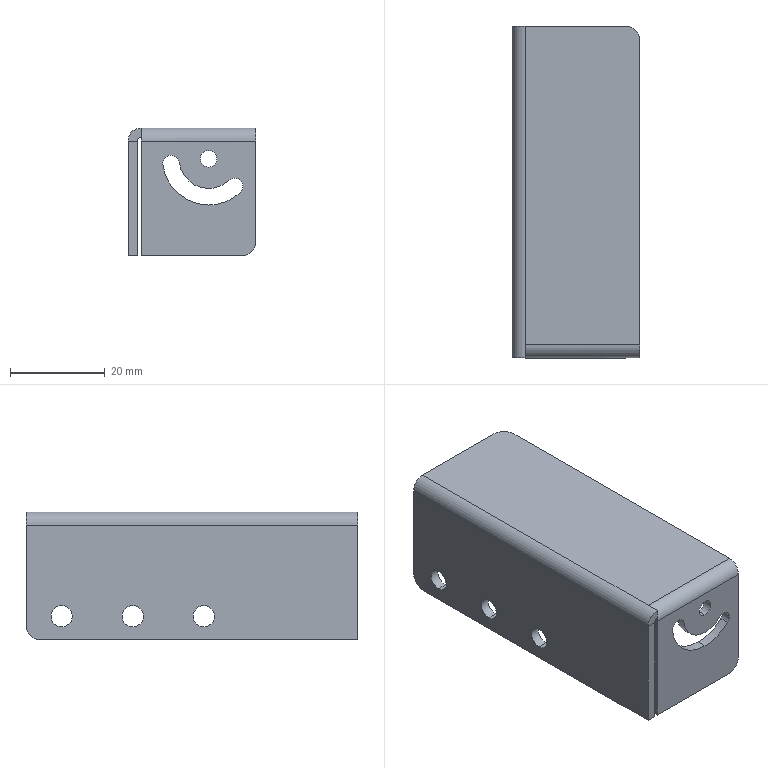Part | SolidWorks | features HoleWzd 2, EdgeFlange 1, Fillet 1, FlatPattern 1, ICE 1, SMBaseFlange 1, SheetMetal 1 | 1 solid | 40 faces | box 27 x 70 x 27 mm | volume 8082 mm3 | cylinder 21 | plane 19 | commonest cylinder face diameters 4.5 x6 3.5 x4 6 x3 1.5 x2 5.5 x2 12.5 x2
STEP:
#1=CARTESIAN_POINT('',(15.,2.,-14.25));
#2=VERTEX_POINT('',#1);
#3=CARTESIAN_POINT('',(21.703,2.,-11.58));
#4=VERTEX_POINT('',#3);
#5=CARTESIAN_POINT('',(15.,2.,-4.5));
#6=DIRECTION('',(0.,-1.,0.));
#7=DIRECTION('',(0.,0.,-1.));
#8=AXIS2_PLACEMENT_3D('',#5,#6,#7);
#9=CIRCLE('',#8,9.75);
#10=EDGE_CURVE('',#2,#4,#9,.T.);
#11=ORIENTED_EDGE('',*,*,#10,.F.);
#12=CARTESIAN_POINT('',(15.,0.,-14.25));
#13=VERTEX_POINT('',#12);
#14=CARTESIAN_POINT('',(15.,2.,-14.25));
#15=DIRECTION('',(0.,-1.,0.));
#16=VECTOR('',#15,1000.);
#17=LINE('',#14,#16);
#18=EDGE_CURVE('',#2,#13,#17,.T.);
#19=ORIENTED_EDGE('',*,*,#18,.T.);
#20=CARTESIAN_POINT('',(21.703,0.,-11.58));
#21=VERTEX_POINT('',#20);
#22=CARTESIAN_POINT('',(15.,0.,-4.5));
#23=DIRECTION('',(0.,-1.,0.));
#24=DIRECTION('',(0.,0.,-1.));
#25=AXIS2_PLACEMENT_3D('',#22,#23,#24);
#26=CIRCLE('',#25,9.75);
#27=EDGE_CURVE('',#13,#21,#26,.T.);
#28=ORIENTED_EDGE('',*,*,#27,.T.);
#29=CARTESIAN_POINT('',(21.703,2.,-11.58));
#30=DIRECTION('',(0.,-1.,0.));
#31=VECTOR('',#30,1000.);
#32=LINE('',#29,#31);
#33=EDGE_CURVE('',#4,#21,#32,.T.);
#34=ORIENTED_EDGE('',*,*,#33,.F.);
#35=EDGE_LOOP('',(#11,#19,#28,#34));
#36=FACE_OUTER_BOUND('',#35,.T.);
#37=CARTESIAN_POINT('',(15.,2.,-4.5));
#38=DIRECTION('',(0.,-1.,0.));
#39=DIRECTION('',(0.,0.,-1.));
#40=AXIS2_PLACEMENT_3D('',#37,#38,#39);
#41=CYLINDRICAL_SURFACE('',#40,9.75);
#42=ADVANCED_FACE('',(#36),#41,.F.);
#43=CARTESIAN_POINT('',(15.,2.,-10.75));
#44=VERTEX_POINT('',#43);
#45=CARTESIAN_POINT('',(8.799,2.,-5.281));
#46=VERTEX_POINT('',#45);
#47=CARTESIAN_POINT('',(15.,2.,-4.5));
#48=DIRECTION('',(0.,1.,0.));
#49=DIRECTION('',(0.,0.,-1.));
#50=AXIS2_PLACEMENT_3D('',#47,#48,#49);
#51=CIRCLE('',#50,6.25);
#52=EDGE_CURVE('',#44,#46,#51,.T.);
#53=ORIENTED_EDGE('',*,*,#52,.F.);
#54=CARTESIAN_POINT('',(15.,0.,-10.75));
#55=VERTEX_POINT('',#54);
#56=CARTESIAN_POINT('',(15.,2.,-10.75));
#57=DIRECTION('',(0.,-1.,0.));
#58=VECTOR('',#57,1000.);
#59=LINE('',#56,#58);
#60=EDGE_CURVE('',#44,#55,#59,.T.);
#61=ORIENTED_EDGE('',*,*,#60,.T.);
#62=CARTESIAN_POINT('',(8.799,0.,-5.281));
#63=VERTEX_POINT('',#62);
#64=CARTESIAN_POINT('',(15.,0.,-4.5));
#65=DIRECTION('',(0.,1.,0.));
#66=DIRECTION('',(0.,0.,-1.));
#67=AXIS2_PLACEMENT_3D('',#64,#65,#66);
#68=CIRCLE('',#67,6.25);
#69=EDGE_CURVE('',#55,#63,#68,.T.);
#70=ORIENTED_EDGE('',*,*,#69,.T.);
#71=CARTESIAN_POINT('',(8.799,2.,-5.281));
#72=DIRECTION('',(0.,-1.,0.));
#73=VECTOR('',#72,1000.);
#74=LINE('',#71,#73);
#75=EDGE_CURVE('',#46,#63,#74,.T.);
#76=ORIENTED_EDGE('',*,*,#75,.F.);
#77=EDGE_LOOP('',(#53,#61,#70,#76));
#78=FACE_OUTER_BOUND('',#77,.T.);
#79=CARTESIAN_POINT('',(15.,2.,-4.5));
#80=DIRECTION('',(0.,-1.,0.));
#81=DIRECTION('',(0.,0.,-1.));
#82=AXIS2_PLACEMENT_3D('',#79,#80,#81);
#83=CYLINDRICAL_SURFACE('',#82,6.25);
#84=ADVANCED_FACE('',(#78),#83,.T.);
#85=CARTESIAN_POINT('',(-2.,62.5,-17.75));
#86=VERTEX_POINT('',#85);
#87=CARTESIAN_POINT('',(-2.,62.5,-22.25));
#88=VERTEX_POINT('',#87);
#89=CARTESIAN_POINT('',(-2.,62.5,-20.));
#90=DIRECTION('',(1.,0.,0.));
#91=DIRECTION('',(0.,0.,-1.));
#92=AXIS2_PLACEMENT_3D('',#89,#90,#91);
#93=CIRCLE('',#92,2.25);
#94=EDGE_CURVE('',#86,#88,#93,.T.);
#95=ORIENTED_EDGE('',*,*,#94,.F.);
#96=CARTESIAN_POINT('',(0.,62.5,-17.75));
#97=VERTEX_POINT('',#96);
#98=CARTESIAN_POINT('',(0.,62.5,-17.75));
#99=DIRECTION('',(1.,0.,0.));
#100=VECTOR('',#99,1000.);
#101=LINE('',#98,#100);
#102=EDGE_CURVE('',#86,#97,#101,.T.);
#103=ORIENTED_EDGE('',*,*,#102,.T.);
#104=CARTESIAN_POINT('',(0.,62.5,-22.25));
#105=VERTEX_POINT('',#104);
#106=CARTESIAN_POINT('',(0.,62.5,-20.));
#107=DIRECTION('',(1.,0.,0.));
#108=DIRECTION('',(0.,0.,-1.));
#109=AXIS2_PLACEMENT_3D('',#106,#107,#108);
#110=CIRCLE('',#109,2.25);
#111=EDGE_CURVE('',#97,#105,#110,.T.);
#112=ORIENTED_EDGE('',*,*,#111,.T.);
#113=CARTESIAN_POINT('',(0.,62.5,-22.25));
#114=DIRECTION('',(1.,0.,0.));
#115=VECTOR('',#114,1000.);
#116=LINE('',#113,#115);
#117=EDGE_CURVE('',#88,#105,#116,.T.);
#118=ORIENTED_EDGE('',*,*,#117,.F.);
#119=EDGE_LOOP('',(#95,#103,#112,#118));
#120=FACE_OUTER_BOUND('',#119,.T.);
#121=CARTESIAN_POINT('',(0.,62.5,-20.));
#122=DIRECTION('',(1.,0.,0.));
#123=DIRECTION('',(0.,0.,-1.));
#124=AXIS2_PLACEMENT_3D('',#121,#122,#123);
#125=CYLINDRICAL_SURFACE('',#124,2.25);
#126=ADVANCED_FACE('',(#120),#125,.F.);
#127=CARTESIAN_POINT('',(-2.,47.5,-17.75));
#128=VERTEX_POINT('',#127);
#129=CARTESIAN_POINT('',(-2.,47.5,-22.25));
#130=VERTEX_POINT('',#129);
#131=CARTESIAN_POINT('',(-2.,47.5,-20.));
#132=DIRECTION('',(1.,0.,0.));
#133=DIRECTION('',(0.,0.,-1.));
#134=AXIS2_PLACEMENT_3D('',#131,#132,#133);
#135=CIRCLE('',#134,2.25);
#136=EDGE_CURVE('',#128,#130,#135,.T.);
#137=ORIENTED_EDGE('',*,*,#136,.F.);
#138=CARTESIAN_POINT('',(0.,47.5,-17.75));
#139=VERTEX_POINT('',#138);
#140=CARTESIAN_POINT('',(0.,47.5,-17.75));
#141=DIRECTION('',(1.,0.,0.));
#142=VECTOR('',#141,1000.);
#143=LINE('',#140,#142);
#144=EDGE_CURVE('',#128,#139,#143,.T.);
#145=ORIENTED_EDGE('',*,*,#144,.T.);
#146=CARTESIAN_POINT('',(0.,47.5,-22.25));
#147=VERTEX_POINT('',#146);
#148=CARTESIAN_POINT('',(0.,47.5,-20.));
#149=DIRECTION('',(1.,0.,0.));
#150=DIRECTION('',(0.,0.,-1.));
#151=AXIS2_PLACEMENT_3D('',#148,#149,#150);
#152=CIRCLE('',#151,2.25);
#153=EDGE_CURVE('',#139,#147,#152,.T.);
#154=ORIENTED_EDGE('',*,*,#153,.T.);
#155=CARTESIAN_POINT('',(0.,47.5,-22.25));
#156=DIRECTION('',(1.,0.,0.));
#157=VECTOR('',#156,1000.);
#158=LINE('',#155,#157);
#159=EDGE_CURVE('',#130,#147,#158,.T.);
#160=ORIENTED_EDGE('',*,*,#159,.F.);
#161=EDGE_LOOP('',(#137,#145,#154,#160));
#162=FACE_OUTER_BOUND('',#161,.T.);
#163=CARTESIAN_POINT('',(0.,47.5,-20.));
#164=DIRECTION('',(1.,0.,0.));
#165=DIRECTION('',(0.,0.,-1.));
#166=AXIS2_PLACEMENT_3D('',#163,#164,#165);
#167=CYLINDRICAL_SURFACE('',#166,2.25);
#168=ADVANCED_FACE('',(#162),#167,.F.);
#169=CARTESIAN_POINT('',(-2.,32.5,-17.75));
#170=VERTEX_POINT('',#169);
#171=CARTESIAN_POINT('',(-2.,32.5,-22.25));
#172=VERTEX_POINT('',#171);
#173=CARTESIAN_POINT('',(-2.,32.5,-20.));
#174=DIRECTION('',(1.,0.,0.));
#175=DIRECTION('',(0.,0.,-1.));
#176=AXIS2_PLACEMENT_3D('',#173,#174,#175);
#177=CIRCLE('',#176,2.25);
#178=EDGE_CURVE('',#170,#172,#177,.T.);
#179=ORIENTED_EDGE('',*,*,#178,.F.);
#180=CARTESIAN_POINT('',(0.,32.5,-17.75));
#181=VERTEX_POINT('',#180);
#182=CARTESIAN_POINT('',(0.,32.5,-17.75));
#183=DIRECTION('',(1.,0.,0.));
#184=VECTOR('',#183,1000.);
#185=LINE('',#182,#184);
#186=EDGE_CURVE('',#170,#181,#185,.T.);
#187=ORIENTED_EDGE('',*,*,#186,.T.);
#188=CARTESIAN_POINT('',(0.,32.5,-22.25));
#189=VERTEX_POINT('',#188);
#190=CARTESIAN_POINT('',(0.,32.5,-20.));
#191=DIRECTION('',(1.,0.,0.));
#192=DIRECTION('',(0.,0.,-1.));
#193=AXIS2_PLACEMENT_3D('',#190,#191,#192);
#194=CIRCLE('',#193,2.25);
#195=EDGE_CURVE('',#181,#189,#194,.T.);
#196=ORIENTED_EDGE('',*,*,#195,.T.);
#197=CARTESIAN_POINT('',(0.,32.5,-22.25));
#198=DIRECTION('',(1.,0.,0.));
#199=VECTOR('',#198,1000.);
#200=LINE('',#197,#199);
#201=EDGE_CURVE('',#172,#189,#200,.T.);
#202=ORIENTED_EDGE('',*,*,#201,.F.);
#203=EDGE_LOOP('',(#179,#187,#196,#202));
#204=FACE_OUTER_BOUND('',#203,.T.);
#205=CARTESIAN_POINT('',(0.,32.5,-20.));
#206=DIRECTION('',(1.,0.,0.));
#207=DIRECTION('',(0.,0.,-1.));
#208=AXIS2_PLACEMENT_3D('',#205,#206,#207);
#209=CYLINDRICAL_SURFACE('',#208,2.25);
#210=ADVANCED_FACE('',(#204),#209,.F.);
#211=CARTESIAN_POINT('',(15.,0.,-2.75));
#212=VERTEX_POINT('',#211);
#213=CARTESIAN_POINT('',(15.,0.,-6.25));
#214=VERTEX_POINT('',#213);
#215=CARTESIAN_POINT('',(15.,0.,-4.5));
#216=DIRECTION('',(0.,-1.,0.));
#217=DIRECTION('',(0.,0.,-1.));
#218=AXIS2_PLACEMENT_3D('',#215,#216,#217);
#219=CIRCLE('',#218,1.75);
#220=EDGE_CURVE('',#212,#214,#219,.T.);
#221=ORIENTED_EDGE('',*,*,#220,.T.);
#222=CARTESIAN_POINT('',(15.,2.,-6.25));
#223=VERTEX_POINT('',#222);
#224=CARTESIAN_POINT('',(15.,2.,-6.25));
#225=DIRECTION('',(0.,1.,0.));
#226=VECTOR('',#225,1000.);
#227=LINE('',#224,#226);
#228=EDGE_CURVE('',#214,#223,#227,.T.);
#229=ORIENTED_EDGE('',*,*,#228,.T.);
#230=CARTESIAN_POINT('',(15.,2.,-2.75));
#231=VERTEX_POINT('',#230);
#232=CARTESIAN_POINT('',(15.,2.,-4.5));
#233=DIRECTION('',(0.,1.,0.));
#234=DIRECTION('',(0.,0.,1.));
#235=AXIS2_PLACEMENT_3D('',#232,#233,#234);
#236=CIRCLE('',#235,1.75);
#237=EDGE_CURVE('',#223,#231,#236,.T.);
#238=ORIENTED_EDGE('',*,*,#237,.T.);
#239=CARTESIAN_POINT('',(15.,2.,-2.75));
#240=DIRECTION('',(0.,1.,0.));
#241=VECTOR('',#240,1000.);
#242=LINE('',#239,#241);
#243=EDGE_CURVE('',#212,#231,#242,.T.);
#244=ORIENTED_EDGE('',*,*,#243,.F.);
#245=EDGE_LOOP('',(#221,#229,#238,#244));
#246=FACE_OUTER_BOUND('',#245,.T.);
#247=CARTESIAN_POINT('',(15.,2.,-4.5));
#248=DIRECTION('',(0.,1.,0.));
#249=DIRECTION('',(0.,0.,1.));
#250=AXIS2_PLACEMENT_3D('',#247,#248,#249);
#251=CYLINDRICAL_SURFACE('',#250,1.75);
#252=ADVANCED_FACE('',(#246),#251,.F.);
#253=CARTESIAN_POINT('',(0.75,0.,0.));
#254=VERTEX_POINT('',#253);
#255=CARTESIAN_POINT('',(0.75,0.1042,0.));
#256=VERTEX_POINT('',#255);
#257=CARTESIAN_POINT('',(0.75,0.,0.));
#258=DIRECTION('',(0.,1.,0.));
#259=VECTOR('',#258,1000.);
#260=LINE('',#257,#259);
#261=EDGE_CURVE('',#254,#256,#260,.T.);
#262=ORIENTED_EDGE('',*,*,#261,.T.);
#263=CARTESIAN_POINT('',(0.75,2.75,2.));
#264=VERTEX_POINT('',#263);
#265=CARTESIAN_POINT('',(0.75,2.75,-0.75));
#266=DIRECTION('',(-1.,0.,0.));
#267=DIRECTION('',(0.,0.,1.));
#268=AXIS2_PLACEMENT_3D('',#265,#266,#267);
#269=CIRCLE('',#268,2.75);
#270=EDGE_CURVE('',#256,#264,#269,.T.);
#271=ORIENTED_EDGE('',*,*,#270,.T.);
#272=CARTESIAN_POINT('',(0.75,0.,2.));
#273=VERTEX_POINT('',#272);
#274=CARTESIAN_POINT('',(0.75,70.,2.));
#275=DIRECTION('',(0.,-1.,0.));
#276=VECTOR('',#275,1000.);
#277=LINE('',#274,#276);
#278=EDGE_CURVE('',#264,#273,#277,.T.);
#279=ORIENTED_EDGE('',*,*,#278,.T.);
#280=CARTESIAN_POINT('',(0.75,0.,2.));
#281=DIRECTION('',(0.,0.,-1.));
#282=VECTOR('',#281,1000.);
#283=LINE('',#280,#282);
#284=EDGE_CURVE('',#273,#254,#283,.T.);
#285=ORIENTED_EDGE('',*,*,#284,.T.);
#286=EDGE_LOOP('',(#262,#271,#279,#285));
#287=FACE_OUTER_BOUND('',#286,.T.);
#288=CARTESIAN_POINT('',(0.75,0.,0.));
#289=DIRECTION('',(1.,0.,0.));
#290=DIRECTION('',(0.,1.,0.));
#291=AXIS2_PLACEMENT_3D('',#288,#289,#290);
#292=PLANE('',#291);
#293=ADVANCED_FACE('',(#287),#292,.T.);
#294=CARTESIAN_POINT('',(25.,67.,2.));
#295=VERTEX_POINT('',#294);
#296=CARTESIAN_POINT('',(25.,2.75,2.));
#297=VERTEX_POINT('',#296);
#298=CARTESIAN_POINT('',(25.,70.,2.));
#299=DIRECTION('',(0.,-1.,0.));
#300=VECTOR('',#299,1000.);
#301=LINE('',#298,#300);
#302=EDGE_CURVE('',#295,#297,#301,.T.);
#303=ORIENTED_EDGE('',*,*,#302,.F.);
#304=CARTESIAN_POINT('',(22.,70.,2.));
#305=VERTEX_POINT('',#304);
#306=CARTESIAN_POINT('',(22.,67.,2.));
#307=DIRECTION('',(0.,0.,1.));
#308=DIRECTION('',(-1.,0.,0.));
#309=AXIS2_PLACEMENT_3D('',#306,#307,#308);
#310=CIRCLE('',#309,3.);
#311=EDGE_CURVE('',#295,#305,#310,.T.);
#312=ORIENTED_EDGE('',*,*,#311,.T.);
#313=CARTESIAN_POINT('',(0.75,70.,2.));
#314=VERTEX_POINT('',#313);
#315=CARTESIAN_POINT('',(0.,70.,2.));
#316=DIRECTION('',(1.,0.,0.));
#317=VECTOR('',#316,1000.);
#318=LINE('',#315,#317);
#319=EDGE_CURVE('',#314,#305,#318,.T.);
#320=ORIENTED_EDGE('',*,*,#319,.F.);
#321=CARTESIAN_POINT('',(0.75,70.,2.));
#322=DIRECTION('',(0.,-1.,0.));
#323=VECTOR('',#322,1000.);
#324=LINE('',#321,#323);
#325=EDGE_CURVE('',#314,#264,#324,.T.);
#326=ORIENTED_EDGE('',*,*,#325,.T.);
#327=CARTESIAN_POINT('',(0.75,2.75,2.));
#328=DIRECTION('',(1.,0.,0.));
#329=VECTOR('',#328,1000.);
#330=LINE('',#327,#329);
#331=EDGE_CURVE('',#264,#297,#330,.T.);
#332=ORIENTED_EDGE('',*,*,#331,.T.);
#333=EDGE_LOOP('',(#303,#312,#320,#326,#332));
#334=FACE_OUTER_BOUND('',#333,.T.);
#335=CARTESIAN_POINT('',(0.,70.,2.));
#336=DIRECTION('',(0.,0.,-1.));
#337=DIRECTION('',(-1.,0.,0.));
#338=AXIS2_PLACEMENT_3D('',#335,#336,#337);
#339=PLANE('',#338);
#340=ADVANCED_FACE('',(#334),#339,.F.);
#341=CARTESIAN_POINT('',(0.75,70.,0.));
#342=VERTEX_POINT('',#341);
#343=CARTESIAN_POINT('',(22.,70.,0.));
#344=VERTEX_POINT('',#343);
#345=CARTESIAN_POINT('',(0.,70.,0.));
#346=DIRECTION('',(1.,0.,0.));
#347=VECTOR('',#346,1000.);
#348=LINE('',#345,#347);
#349=EDGE_CURVE('',#342,#344,#348,.T.);
#350=ORIENTED_EDGE('',*,*,#349,.T.);
#351=CARTESIAN_POINT('',(25.,67.,0.));
#352=VERTEX_POINT('',#351);
#353=CARTESIAN_POINT('',(22.,67.,0.));
#354=DIRECTION('',(0.,0.,-1.));
#355=DIRECTION('',(-1.,0.,0.));
#356=AXIS2_PLACEMENT_3D('',#353,#354,#355);
#357=CIRCLE('',#356,3.);
#358=EDGE_CURVE('',#344,#352,#357,.T.);
#359=ORIENTED_EDGE('',*,*,#358,.T.);
#360=CARTESIAN_POINT('',(25.,2.75,0.));
#361=VERTEX_POINT('',#360);
#362=CARTESIAN_POINT('',(25.,70.,0.));
#363=DIRECTION('',(0.,-1.,0.));
#364=VECTOR('',#363,1000.);
#365=LINE('',#362,#364);
#366=EDGE_CURVE('',#352,#361,#365,.T.);
#367=ORIENTED_EDGE('',*,*,#366,.T.);
#368=CARTESIAN_POINT('',(0.75,2.75,0.));
#369=VERTEX_POINT('',#368);
#370=CARTESIAN_POINT('',(0.75,2.75,0.));
#371=DIRECTION('',(1.,0.,0.));
#372=VECTOR('',#371,1000.);
#373=LINE('',#370,#372);
#374=EDGE_CURVE('',#369,#361,#373,.T.);
#375=ORIENTED_EDGE('',*,*,#374,.F.);
#376=CARTESIAN_POINT('',(0.75,70.,0.));
#377=DIRECTION('',(0.,-1.,0.));
#378=VECTOR('',#377,1000.);
#379=LINE('',#376,#378);
#380=EDGE_CURVE('',#342,#369,#379,.T.);
#381=ORIENTED_EDGE('',*,*,#380,.F.);
#382=EDGE_LOOP('',(#350,#359,#367,#375,#381));
#383=FACE_OUTER_BOUND('',#382,.T.);
#384=CARTESIAN_POINT('',(0.,70.,0.));
#385=DIRECTION('',(0.,0.,-1.));
#386=DIRECTION('',(-1.,0.,0.));
#387=AXIS2_PLACEMENT_3D('',#384,#385,#386);
#388=PLANE('',#387);
#389=ADVANCED_FACE('',(#383),#388,.T.);
#390=CARTESIAN_POINT('',(0.75,70.,0.));
#391=DIRECTION('',(0.,0.,1.));
#392=VECTOR('',#391,1000.);
#393=LINE('',#390,#392);
#394=EDGE_CURVE('',#342,#314,#393,.T.);
#395=ORIENTED_EDGE('',*,*,#394,.F.);
#396=CARTESIAN_POINT('',(0.,70.,-0.75));
#397=VERTEX_POINT('',#396);
#398=CARTESIAN_POINT('',(0.75,70.,-0.75));
#399=DIRECTION('',(0.,1.,0.));
#400=DIRECTION('',(0.,0.,-1.));
#401=AXIS2_PLACEMENT_3D('',#398,#399,#400);
#402=CIRCLE('',#401,0.75);
#403=EDGE_CURVE('',#397,#342,#402,.T.);
#404=ORIENTED_EDGE('',*,*,#403,.F.);
#405=CARTESIAN_POINT('',(-2.,70.,-0.75));
#406=VERTEX_POINT('',#405);
#407=CARTESIAN_POINT('',(-2.,70.,-0.75));
#408=DIRECTION('',(1.,0.,0.));
#409=VECTOR('',#408,1000.);
#410=LINE('',#407,#409);
#411=EDGE_CURVE('',#406,#397,#410,.T.);
#412=ORIENTED_EDGE('',*,*,#411,.F.);
#413=CARTESIAN_POINT('',(0.75,70.,-0.75));
#414=DIRECTION('',(0.,1.,0.));
#415=DIRECTION('',(1.,0.,0.));
#416=AXIS2_PLACEMENT_3D('',#413,#414,#415);
#417=CIRCLE('',#416,2.75);
#418=EDGE_CURVE('',#406,#314,#417,.T.);
#419=ORIENTED_EDGE('',*,*,#418,.T.);
#420=EDGE_LOOP('',(#395,#404,#412,#419));
#421=FACE_OUTER_BOUND('',#420,.T.);
#422=CARTESIAN_POINT('',(0.75,70.,0.));
#423=DIRECTION('',(0.,1.,0.));
#424=DIRECTION('',(0.,0.,1.));
#425=AXIS2_PLACEMENT_3D('',#422,#423,#424);
#426=PLANE('',#425);
#427=ADVANCED_FACE('',(#421),#426,.T.);
#428=ORIENTED_EDGE('',*,*,#319,.T.);
#429=CARTESIAN_POINT('',(22.,70.,-0.75));
#430=DIRECTION('',(0.,0.,-1.));
#431=VECTOR('',#430,1000.);
#432=LINE('',#429,#431);
#433=EDGE_CURVE('',#305,#344,#432,.T.);
#434=ORIENTED_EDGE('',*,*,#433,.T.);
#435=ORIENTED_EDGE('',*,*,#349,.F.);
#436=ORIENTED_EDGE('',*,*,#394,.T.);
#437=EDGE_LOOP('',(#428,#434,#435,#436));
#438=FACE_OUTER_BOUND('',#437,.T.);
#439=CARTESIAN_POINT('',(-2.,70.,-0.75));
#440=DIRECTION('',(0.,1.,0.));
#441=DIRECTION('',(0.,0.,1.));
#442=AXIS2_PLACEMENT_3D('',#439,#440,#441);
#443=PLANE('',#442);
#444=ADVANCED_FACE('',(#438),#443,.T.);
#445=CARTESIAN_POINT('',(0.,0.,-0.75));
#446=VERTEX_POINT('',#445);
#447=CARTESIAN_POINT('',(-2.,0.,-0.75));
#448=VERTEX_POINT('',#447);
#449=CARTESIAN_POINT('',(0.,0.,-0.75));
#450=DIRECTION('',(-1.,0.,0.));
#451=VECTOR('',#450,1000.);
#452=LINE('',#449,#451);
#453=EDGE_CURVE('',#446,#448,#452,.T.);
#454=ORIENTED_EDGE('',*,*,#453,.F.);
#455=CARTESIAN_POINT('',(0.75,0.,-0.75));
#456=DIRECTION('',(0.,1.,0.));
#457=DIRECTION('',(0.,0.,-1.));
#458=AXIS2_PLACEMENT_3D('',#455,#456,#457);
#459=CIRCLE('',#458,0.75);
#460=EDGE_CURVE('',#446,#254,#459,.T.);
#461=ORIENTED_EDGE('',*,*,#460,.T.);
#462=ORIENTED_EDGE('',*,*,#284,.F.);
#463=CARTESIAN_POINT('',(0.75,0.,-0.75));
#464=DIRECTION('',(0.,1.,0.));
#465=DIRECTION('',(1.,0.,0.));
#466=AXIS2_PLACEMENT_3D('',#463,#464,#465);
#467=CIRCLE('',#466,2.75);
#468=EDGE_CURVE('',#448,#273,#467,.T.);
#469=ORIENTED_EDGE('',*,*,#468,.F.);
#470=EDGE_LOOP('',(#454,#461,#462,#469));
#471=FACE_OUTER_BOUND('',#470,.T.);
#472=CARTESIAN_POINT('',(0.,0.,-0.75));
#473=DIRECTION('',(0.,-1.,0.));
#474=DIRECTION('',(0.,0.,-1.));
#475=AXIS2_PLACEMENT_3D('',#472,#473,#474);
#476=PLANE('',#475);
#477=ADVANCED_FACE('',(#471),#476,.T.);
#478=CARTESIAN_POINT('',(0.,0.,-25.));
#479=VERTEX_POINT('',#478);
#480=CARTESIAN_POINT('',(0.,0.,-25.));
#481=DIRECTION('',(0.,0.,1.));
#482=VECTOR('',#481,1000.);
#483=LINE('',#480,#482);
#484=EDGE_CURVE('',#479,#446,#483,.T.);
#485=ORIENTED_EDGE('',*,*,#484,.T.);
#486=ORIENTED_EDGE('',*,*,#453,.T.);
#487=CARTESIAN_POINT('',(-2.,0.,-25.));
#488=VERTEX_POINT('',#487);
#489=CARTESIAN_POINT('',(-2.,0.,-25.));
#490=DIRECTION('',(0.,0.,1.));
#491=VECTOR('',#490,1000.);
#492=LINE('',#489,#491);
#493=EDGE_CURVE('',#488,#448,#492,.T.);
#494=ORIENTED_EDGE('',*,*,#493,.F.);
#495=CARTESIAN_POINT('',(-2.,0.,-25.));
#496=DIRECTION('',(1.,0.,0.));
#497=VECTOR('',#496,1000.);
#498=LINE('',#495,#497);
#499=EDGE_CURVE('',#488,#479,#498,.T.);
#500=ORIENTED_EDGE('',*,*,#499,.T.);
#501=EDGE_LOOP('',(#485,#486,#494,#500));
#502=FACE_OUTER_BOUND('',#501,.T.);
#503=CARTESIAN_POINT('',(0.75,0.,2.));
#504=DIRECTION('',(0.,-1.,0.));
#505=DIRECTION('',(0.,0.,-1.));
#506=AXIS2_PLACEMENT_3D('',#503,#504,#505);
#507=PLANE('',#506);
#508=ADVANCED_FACE('',(#502),#507,.T.);
#509=ORIENTED_EDGE('',*,*,#366,.F.);
#510=CARTESIAN_POINT('',(25.,67.,0.));
#511=DIRECTION('',(0.,0.,1.));
#512=VECTOR('',#511,1000.);
#513=LINE('',#510,#512);
#514=EDGE_CURVE('',#352,#295,#513,.T.);
#515=ORIENTED_EDGE('',*,*,#514,.T.);
#516=ORIENTED_EDGE('',*,*,#302,.T.);
#517=CARTESIAN_POINT('',(25.,2.75,0.));
#518=DIRECTION('',(0.,0.,1.));
#519=VECTOR('',#518,1000.);
#520=LINE('',#517,#519);
#521=EDGE_CURVE('',#361,#297,#520,.T.);
#522=ORIENTED_EDGE('',*,*,#521,.F.);
#523=EDGE_LOOP('',(#509,#515,#516,#522));
#524=FACE_OUTER_BOUND('',#523,.T.);
#525=CARTESIAN_POINT('',(25.,70.,0.));
#526=DIRECTION('',(1.,0.,0.));
#527=DIRECTION('',(0.,0.,-1.));
#528=AXIS2_PLACEMENT_3D('',#525,#526,#527);
#529=PLANE('',#528);
#530=ADVANCED_FACE('',(#524),#529,.T.);
#531=ORIENTED_EDGE('',*,*,#460,.F.);
#532=CARTESIAN_POINT('',(0.,70.,-0.75));
#533=DIRECTION('',(0.,-1.,0.));
#534=VECTOR('',#533,1000.);
#535=LINE('',#532,#534);
#536=EDGE_CURVE('',#397,#446,#535,.T.);
#537=ORIENTED_EDGE('',*,*,#536,.F.);
#538=ORIENTED_EDGE('',*,*,#403,.T.);
#539=ORIENTED_EDGE('',*,*,#380,.T.);
#540=CARTESIAN_POINT('',(0.75,0.,0.));
#541=DIRECTION('',(0.,1.,0.));
#542=VECTOR('',#541,1000.);
#543=LINE('',#540,#542);
#544=EDGE_CURVE('',#256,#369,#543,.T.);
#545=ORIENTED_EDGE('',*,*,#544,.F.);
#546=ORIENTED_EDGE('',*,*,#261,.F.);
#547=EDGE_LOOP('',(#531,#537,#538,#539,#545,#546));
#548=FACE_OUTER_BOUND('',#547,.T.);
#549=CARTESIAN_POINT('',(0.75,70.,-0.75));
#550=DIRECTION('',(0.,-1.,0.));
#551=DIRECTION('',(0.,0.,-1.));
#552=AXIS2_PLACEMENT_3D('',#549,#550,#551);
#553=CYLINDRICAL_SURFACE('',#552,0.75);
#554=ADVANCED_FACE('',(#548),#553,.F.);
#555=CARTESIAN_POINT('',(0.,62.5,-20.));
#556=DIRECTION('',(1.,0.,0.));
#557=DIRECTION('',(0.,0.,-1.));
#558=AXIS2_PLACEMENT_3D('',#555,#556,#557);
#559=CIRCLE('',#558,2.25);
#560=EDGE_CURVE('',#105,#97,#559,.T.);
#561=ORIENTED_EDGE('',*,*,#560,.F.);
#562=ORIENTED_EDGE('',*,*,#111,.F.);
#563=EDGE_LOOP('',(#561,#562));
#564=FACE_BOUND('',#563,.T.);
#565=CARTESIAN_POINT('',(0.,47.5,-20.));
#566=DIRECTION('',(1.,0.,0.));
#567=DIRECTION('',(0.,0.,-1.));
#568=AXIS2_PLACEMENT_3D('',#565,#566,#567);
#569=CIRCLE('',#568,2.25);
#570=EDGE_CURVE('',#147,#139,#569,.T.);
#571=ORIENTED_EDGE('',*,*,#570,.F.);
#572=ORIENTED_EDGE('',*,*,#153,.F.);
#573=EDGE_LOOP('',(#571,#572));
#574=FACE_BOUND('',#573,.T.);
#575=CARTESIAN_POINT('',(0.,32.5,-20.));
#576=DIRECTION('',(1.,0.,0.));
#577=DIRECTION('',(0.,0.,-1.));
#578=AXIS2_PLACEMENT_3D('',#575,#576,#577);
#579=CIRCLE('',#578,2.25);
#580=EDGE_CURVE('',#189,#181,#579,.T.);
#581=ORIENTED_EDGE('',*,*,#580,.F.);
#582=ORIENTED_EDGE('',*,*,#195,.F.);
#583=EDGE_LOOP('',(#581,#582));
#584=FACE_BOUND('',#583,.T.);
#585=CARTESIAN_POINT('',(0.,67.,-25.));
#586=VERTEX_POINT('',#585);
#587=CARTESIAN_POINT('',(0.,70.,-25.));
#588=DIRECTION('',(0.,-1.,0.));
#589=VECTOR('',#588,1000.);
#590=LINE('',#587,#589);
#591=EDGE_CURVE('',#586,#479,#590,.T.);
#592=ORIENTED_EDGE('',*,*,#591,.F.);
#593=CARTESIAN_POINT('',(0.,70.,-22.));
#594=VERTEX_POINT('',#593);
#595=CARTESIAN_POINT('',(0.,67.,-22.));
#596=DIRECTION('',(1.,0.,0.));
#597=DIRECTION('',(0.,0.,-1.));
#598=AXIS2_PLACEMENT_3D('',#595,#596,#597);
#599=CIRCLE('',#598,3.);
#600=EDGE_CURVE('',#586,#594,#599,.T.);
#601=ORIENTED_EDGE('',*,*,#600,.T.);
#602=CARTESIAN_POINT('',(0.,70.,-25.));
#603=DIRECTION('',(0.,0.,1.));
#604=VECTOR('',#603,1000.);
#605=LINE('',#602,#604);
#606=EDGE_CURVE('',#594,#397,#605,.T.);
#607=ORIENTED_EDGE('',*,*,#606,.T.);
#608=ORIENTED_EDGE('',*,*,#536,.T.);
#609=ORIENTED_EDGE('',*,*,#484,.F.);
#610=EDGE_LOOP('',(#592,#601,#607,#608,#609));
#611=FACE_OUTER_BOUND('',#610,.T.);
#612=CARTESIAN_POINT('',(0.,70.,-25.));
#613=DIRECTION('',(1.,0.,0.));
#614=DIRECTION('',(0.,0.,-1.));
#615=AXIS2_PLACEMENT_3D('',#612,#613,#614);
#616=PLANE('',#615);
#617=ADVANCED_FACE('',(#564,#574,#584,#611),#616,.T.);
#618=CARTESIAN_POINT('',(-2.,67.,-25.));
#619=VERTEX_POINT('',#618);
#620=CARTESIAN_POINT('',(-2.,70.,-25.));
#621=DIRECTION('',(0.,-1.,0.));
#622=VECTOR('',#621,1000.);
#623=LINE('',#620,#622);
#624=EDGE_CURVE('',#619,#488,#623,.T.);
#625=ORIENTED_EDGE('',*,*,#624,.F.);
#626=CARTESIAN_POINT('',(0.,67.,-25.));
#627=DIRECTION('',(1.,0.,0.));
#628=VECTOR('',#627,1000.);
#629=LINE('',#626,#628);
#630=EDGE_CURVE('',#619,#586,#629,.T.);
#631=ORIENTED_EDGE('',*,*,#630,.T.);
#632=ORIENTED_EDGE('',*,*,#591,.T.);
#633=ORIENTED_EDGE('',*,*,#499,.F.);
#634=EDGE_LOOP('',(#625,#631,#632,#633));
#635=FACE_OUTER_BOUND('',#634,.T.);
#636=CARTESIAN_POINT('',(-2.,70.,-25.));
#637=DIRECTION('',(0.,0.,-1.));
#638=DIRECTION('',(-1.,0.,0.));
#639=AXIS2_PLACEMENT_3D('',#636,#637,#638);
#640=PLANE('',#639);
#641=ADVANCED_FACE('',(#635),#640,.T.);
#642=CARTESIAN_POINT('',(-2.,62.5,-20.));
#643=DIRECTION('',(1.,0.,0.));
#644=DIRECTION('',(0.,0.,-1.));
#645=AXIS2_PLACEMENT_3D('',#642,#643,#644);
#646=CIRCLE('',#645,2.25);
#647=EDGE_CURVE('',#88,#86,#646,.T.);
#648=ORIENTED_EDGE('',*,*,#647,.T.);
#649=ORIENTED_EDGE('',*,*,#94,.T.);
#650=EDGE_LOOP('',(#648,#649));
#651=FACE_BOUND('',#650,.T.);
#652=CARTESIAN_POINT('',(-2.,47.5,-20.));
#653=DIRECTION('',(1.,0.,0.));
#654=DIRECTION('',(0.,0.,-1.));
#655=AXIS2_PLACEMENT_3D('',#652,#653,#654);
#656=CIRCLE('',#655,2.25);
#657=EDGE_CURVE('',#130,#128,#656,.T.);
#658=ORIENTED_EDGE('',*,*,#657,.T.);
#659=ORIENTED_EDGE('',*,*,#136,.T.);
#660=EDGE_LOOP('',(#658,#659));
#661=FACE_BOUND('',#660,.T.);
#662=CARTESIAN_POINT('',(-2.,32.5,-20.));
#663=DIRECTION('',(1.,0.,0.));
#664=DIRECTION('',(0.,0.,-1.));
#665=AXIS2_PLACEMENT_3D('',#662,#663,#664);
#666=CIRCLE('',#665,2.25);
#667=EDGE_CURVE('',#172,#170,#666,.T.);
#668=ORIENTED_EDGE('',*,*,#667,.T.);
#669=ORIENTED_EDGE('',*,*,#178,.T.);
#670=EDGE_LOOP('',(#668,#669));
#671=FACE_BOUND('',#670,.T.);
#672=CARTESIAN_POINT('',(-2.,70.,-22.));
#673=VERTEX_POINT('',#672);
#674=CARTESIAN_POINT('',(-2.,70.,-25.));
#675=DIRECTION('',(0.,0.,1.));
#676=VECTOR('',#675,1000.);
#677=LINE('',#674,#676);
#678=EDGE_CURVE('',#673,#406,#677,.T.);
#679=ORIENTED_EDGE('',*,*,#678,.F.);
#680=CARTESIAN_POINT('',(-2.,67.,-22.));
#681=DIRECTION('',(-1.,0.,0.));
#682=DIRECTION('',(0.,0.,-1.));
#683=AXIS2_PLACEMENT_3D('',#680,#681,#682);
#684=CIRCLE('',#683,3.);
#685=EDGE_CURVE('',#673,#619,#684,.T.);
#686=ORIENTED_EDGE('',*,*,#685,.T.);
#687=ORIENTED_EDGE('',*,*,#624,.T.);
#688=ORIENTED_EDGE('',*,*,#493,.T.);
#689=CARTESIAN_POINT('',(-2.,70.,-0.75));
#690=DIRECTION('',(0.,-1.,0.));
#691=VECTOR('',#690,1000.);
#692=LINE('',#689,#691);
#693=EDGE_CURVE('',#406,#448,#692,.T.);
#694=ORIENTED_EDGE('',*,*,#693,.F.);
#695=EDGE_LOOP('',(#679,#686,#687,#688,#694));
#696=FACE_OUTER_BOUND('',#695,.T.);
#697=CARTESIAN_POINT('',(-2.,70.,-25.));
#698=DIRECTION('',(1.,0.,0.));
#699=DIRECTION('',(0.,0.,-1.));
#700=AXIS2_PLACEMENT_3D('',#697,#698,#699);
#701=PLANE('',#700);
#702=ADVANCED_FACE('',(#651,#661,#671,#696),#701,.F.);
#703=ORIENTED_EDGE('',*,*,#468,.T.);
#704=ORIENTED_EDGE('',*,*,#278,.F.);
#705=ORIENTED_EDGE('',*,*,#325,.F.);
#706=ORIENTED_EDGE('',*,*,#418,.F.);
#707=ORIENTED_EDGE('',*,*,#693,.T.);
#708=EDGE_LOOP('',(#703,#704,#705,#706,#707));
#709=FACE_OUTER_BOUND('',#708,.T.);
#710=CARTESIAN_POINT('',(0.75,70.,-0.75));
#711=DIRECTION('',(0.,-1.,0.));
#712=DIRECTION('',(0.,0.,-1.));
#713=AXIS2_PLACEMENT_3D('',#710,#711,#712);
#714=CYLINDRICAL_SURFACE('',#713,2.75);
#715=ADVANCED_FACE('',(#709),#714,.T.);
#716=ORIENTED_EDGE('',*,*,#606,.F.);
#717=CARTESIAN_POINT('',(-2.,70.,-22.));
#718=DIRECTION('',(-1.,0.,0.));
#719=VECTOR('',#718,1000.);
#720=LINE('',#717,#719);
#721=EDGE_CURVE('',#594,#673,#720,.T.);
#722=ORIENTED_EDGE('',*,*,#721,.T.);
#723=ORIENTED_EDGE('',*,*,#678,.T.);
#724=ORIENTED_EDGE('',*,*,#411,.T.);
#725=EDGE_LOOP('',(#716,#722,#723,#724));
#726=FACE_OUTER_BOUND('',#725,.T.);
#727=CARTESIAN_POINT('',(0.75,70.,-0.75));
#728=DIRECTION('',(0.,-1.,0.));
#729=DIRECTION('',(-1.,0.,0.));
#730=AXIS2_PLACEMENT_3D('',#727,#728,#729);
#731=PLANE('',#730);
#732=ADVANCED_FACE('',(#726),#731,.F.);
#733=CARTESIAN_POINT('',(25.,2.,-0.75));
#734=VERTEX_POINT('',#733);
#735=CARTESIAN_POINT('',(25.,0.,-0.75));
#736=VERTEX_POINT('',#735);
#737=CARTESIAN_POINT('',(25.,0.,-0.75));
#738=DIRECTION('',(0.,-1.,0.));
#739=VECTOR('',#738,1000.);
#740=LINE('',#737,#739);
#741=EDGE_CURVE('',#734,#736,#740,.T.);
#742=ORIENTED_EDGE('',*,*,#741,.F.);
#743=CARTESIAN_POINT('',(25.,2.75,-0.75));
#744=DIRECTION('',(1.,0.,0.));
#745=DIRECTION('',(0.,0.,1.));
#746=AXIS2_PLACEMENT_3D('',#743,#744,#745);
#747=CIRCLE('',#746,0.75);
#748=EDGE_CURVE('',#361,#734,#747,.T.);
#749=ORIENTED_EDGE('',*,*,#748,.F.);
#750=ORIENTED_EDGE('',*,*,#521,.T.);
#751=CARTESIAN_POINT('',(25.,2.75,-0.75));
#752=DIRECTION('',(1.,0.,0.));
#753=DIRECTION('',(0.,0.,1.));
#754=AXIS2_PLACEMENT_3D('',#751,#752,#753);
#755=CIRCLE('',#754,2.75);
#756=EDGE_CURVE('',#297,#736,#755,.T.);
#757=ORIENTED_EDGE('',*,*,#756,.T.);
#758=EDGE_LOOP('',(#742,#749,#750,#757));
#759=FACE_OUTER_BOUND('',#758,.T.);
#760=CARTESIAN_POINT('',(25.,2.75,-0.75));
#761=DIRECTION('',(1.,0.,0.));
#762=DIRECTION('',(0.,0.,-1.));
#763=AXIS2_PLACEMENT_3D('',#760,#761,#762);
#764=PLANE('',#763);
#765=ADVANCED_FACE('',(#759),#764,.T.);
#766=CARTESIAN_POINT('',(0.75,0.,-0.75));
#767=VERTEX_POINT('',#766);
#768=CARTESIAN_POINT('',(0.75,2.75,-0.75));
#769=DIRECTION('',(-1.,0.,0.));
#770=DIRECTION('',(0.,0.,1.));
#771=AXIS2_PLACEMENT_3D('',#768,#769,#770);
#772=CIRCLE('',#771,2.75);
#773=EDGE_CURVE('',#767,#256,#772,.T.);
#774=ORIENTED_EDGE('',*,*,#773,.T.);
#775=ORIENTED_EDGE('',*,*,#544,.T.);
#776=CARTESIAN_POINT('',(0.75,2.,-0.75));
#777=VERTEX_POINT('',#776);
#778=CARTESIAN_POINT('',(0.75,2.75,-0.75));
#779=DIRECTION('',(-1.,0.,0.));
#780=DIRECTION('',(0.,0.,1.));
#781=AXIS2_PLACEMENT_3D('',#778,#779,#780);
#782=CIRCLE('',#781,0.75);
#783=EDGE_CURVE('',#777,#369,#782,.T.);
#784=ORIENTED_EDGE('',*,*,#783,.F.);
#785=CARTESIAN_POINT('',(0.75,2.,-0.75));
#786=DIRECTION('',(0.,-1.,0.));
#787=VECTOR('',#786,1000.);
#788=LINE('',#785,#787);
#789=EDGE_CURVE('',#777,#767,#788,.T.);
#790=ORIENTED_EDGE('',*,*,#789,.T.);
#791=EDGE_LOOP('',(#774,#775,#784,#790));
#792=FACE_OUTER_BOUND('',#791,.T.);
#793=CARTESIAN_POINT('',(0.75,2.75,-0.75));
#794=DIRECTION('',(1.,0.,0.));
#795=DIRECTION('',(0.,0.,-1.));
#796=AXIS2_PLACEMENT_3D('',#793,#794,#795);
#797=PLANE('',#796);
#798=ADVANCED_FACE('',(#792),#797,.F.);
#799=ORIENTED_EDGE('',*,*,#331,.F.);
#800=ORIENTED_EDGE('',*,*,#270,.F.);
#801=ORIENTED_EDGE('',*,*,#773,.F.);
#802=CARTESIAN_POINT('',(0.,0.,-0.75));
#803=DIRECTION('',(-1.,0.,0.));
#804=VECTOR('',#803,1000.);
#805=LINE('',#802,#804);
#806=EDGE_CURVE('',#736,#767,#805,.T.);
#807=ORIENTED_EDGE('',*,*,#806,.F.);
#808=ORIENTED_EDGE('',*,*,#756,.F.);
#809=EDGE_LOOP('',(#799,#800,#801,#807,#808));
#810=FACE_OUTER_BOUND('',#809,.T.);
#811=CARTESIAN_POINT('',(0.75,2.75,-0.75));
#812=DIRECTION('',(-1.,0.,0.));
#813=DIRECTION('',(0.,-1.,0.));
#814=AXIS2_PLACEMENT_3D('',#811,#812,#813);
#815=CYLINDRICAL_SURFACE('',#814,2.75);
#816=ADVANCED_FACE('',(#810),#815,.T.);
#817=ORIENTED_EDGE('',*,*,#374,.T.);
#818=ORIENTED_EDGE('',*,*,#748,.T.);
#819=CARTESIAN_POINT('',(25.,2.,-0.75));
#820=DIRECTION('',(-1.,0.,0.));
#821=VECTOR('',#820,1000.);
#822=LINE('',#819,#821);
#823=EDGE_CURVE('',#734,#777,#822,.T.);
#824=ORIENTED_EDGE('',*,*,#823,.T.);
#825=ORIENTED_EDGE('',*,*,#783,.T.);
#826=EDGE_LOOP('',(#817,#818,#824,#825));
#827=FACE_OUTER_BOUND('',#826,.T.);
#828=CARTESIAN_POINT('',(0.75,2.75,-0.75));
#829=DIRECTION('',(-1.,0.,0.));
#830=DIRECTION('',(0.,-1.,0.));
#831=AXIS2_PLACEMENT_3D('',#828,#829,#830);
#832=CYLINDRICAL_SURFACE('',#831,0.75);
#833=ADVANCED_FACE('',(#827),#832,.F.);
#834=CARTESIAN_POINT('',(0.75,0.,-25.));
#835=VERTEX_POINT('',#834);
#836=CARTESIAN_POINT('',(0.75,0.,0.));
#837=DIRECTION('',(0.,0.,1.));
#838=VECTOR('',#837,1000.);
#839=LINE('',#836,#838);
#840=EDGE_CURVE('',#835,#767,#839,.T.);
#841=ORIENTED_EDGE('',*,*,#840,.T.);
#842=ORIENTED_EDGE('',*,*,#789,.F.);
#843=CARTESIAN_POINT('',(0.75,2.,-25.));
#844=VERTEX_POINT('',#843);
#845=CARTESIAN_POINT('',(0.75,2.,0.));
#846=DIRECTION('',(0.,0.,1.));
#847=VECTOR('',#846,1000.);
#848=LINE('',#845,#847);
#849=EDGE_CURVE('',#844,#777,#848,.T.);
#850=ORIENTED_EDGE('',*,*,#849,.F.);
#851=CARTESIAN_POINT('',(0.75,0.,-25.));
#852=DIRECTION('',(0.,1.,0.));
#853=VECTOR('',#852,1000.);
#854=LINE('',#851,#853);
#855=EDGE_CURVE('',#835,#844,#854,.T.);
#856=ORIENTED_EDGE('',*,*,#855,.F.);
#857=EDGE_LOOP('',(#841,#842,#850,#856));
#858=FACE_OUTER_BOUND('',#857,.T.);
#859=CARTESIAN_POINT('',(0.75,0.,0.));
#860=DIRECTION('',(-1.,0.,0.));
#861=DIRECTION('',(0.,0.,1.));
#862=AXIS2_PLACEMENT_3D('',#859,#860,#861);
#863=PLANE('',#862);
#864=ADVANCED_FACE('',(#858),#863,.T.);
#865=CARTESIAN_POINT('',(25.,0.,-22.));
#866=VERTEX_POINT('',#865);
#867=CARTESIAN_POINT('',(25.,0.,-25.));
#868=DIRECTION('',(0.,0.,-1.));
#869=VECTOR('',#868,1000.);
#870=LINE('',#867,#869);
#871=EDGE_CURVE('',#736,#866,#870,.T.);
#872=ORIENTED_EDGE('',*,*,#871,.T.);
#873=CARTESIAN_POINT('',(25.,2.,-22.));
#874=VERTEX_POINT('',#873);
#875=CARTESIAN_POINT('',(25.,0.,-22.));
#876=DIRECTION('',(0.,1.,0.));
#877=VECTOR('',#876,1000.);
#878=LINE('',#875,#877);
#879=EDGE_CURVE('',#866,#874,#878,.T.);
#880=ORIENTED_EDGE('',*,*,#879,.T.);
#881=CARTESIAN_POINT('',(25.,2.,0.));
#882=DIRECTION('',(0.,0.,-1.));
#883=VECTOR('',#882,1000.);
#884=LINE('',#881,#883);
#885=EDGE_CURVE('',#734,#874,#884,.T.);
#886=ORIENTED_EDGE('',*,*,#885,.F.);
#887=ORIENTED_EDGE('',*,*,#741,.T.);
#888=EDGE_LOOP('',(#872,#880,#886,#887));
#889=FACE_OUTER_BOUND('',#888,.T.);
#890=CARTESIAN_POINT('',(25.,0.,-25.));
#891=DIRECTION('',(1.,0.,0.));
#892=DIRECTION('',(0.,0.,-1.));
#893=AXIS2_PLACEMENT_3D('',#890,#891,#892);
#894=PLANE('',#893);
#895=ADVANCED_FACE('',(#889),#894,.T.);
#896=CARTESIAN_POINT('',(5.326,0.,-5.719));
#897=VERTEX_POINT('',#896);
#898=CARTESIAN_POINT('',(7.063,0.,-5.5));
#899=DIRECTION('',(0.,-1.,0.));
#900=DIRECTION('',(0.,0.,-1.));
#901=AXIS2_PLACEMENT_3D('',#898,#899,#900);
#902=CIRCLE('',#901,1.75);
#903=EDGE_CURVE('',#63,#897,#902,.T.);
#904=ORIENTED_EDGE('',*,*,#903,.F.);
#905=ORIENTED_EDGE('',*,*,#69,.F.);
#906=CARTESIAN_POINT('',(19.297,0.,-9.039));
#907=VERTEX_POINT('',#906);
#908=CARTESIAN_POINT('',(15.,0.,-4.5));
#909=DIRECTION('',(0.,1.,0.));
#910=DIRECTION('',(0.,0.,-1.));
#911=AXIS2_PLACEMENT_3D('',#908,#909,#910);
#912=CIRCLE('',#911,6.25);
#913=EDGE_CURVE('',#907,#55,#912,.T.);
#914=ORIENTED_EDGE('',*,*,#913,.F.);
#915=CARTESIAN_POINT('',(20.5,0.,-10.309));
#916=DIRECTION('',(0.,-1.,0.));
#917=DIRECTION('',(0.,0.,-1.));
#918=AXIS2_PLACEMENT_3D('',#915,#916,#917);
#919=CIRCLE('',#918,1.75);
#920=EDGE_CURVE('',#21,#907,#919,.T.);
#921=ORIENTED_EDGE('',*,*,#920,.F.);
#922=ORIENTED_EDGE('',*,*,#27,.F.);
#923=CARTESIAN_POINT('',(15.,0.,-4.5));
#924=DIRECTION('',(0.,-1.,0.));
#925=DIRECTION('',(0.,0.,-1.));
#926=AXIS2_PLACEMENT_3D('',#923,#924,#925);
#927=CIRCLE('',#926,9.75);
#928=EDGE_CURVE('',#897,#13,#927,.T.);
#929=ORIENTED_EDGE('',*,*,#928,.F.);
#930=EDGE_LOOP('',(#904,#905,#914,#921,#922,#929));
#931=FACE_BOUND('',#930,.T.);
#932=ORIENTED_EDGE('',*,*,#220,.F.);
#933=CARTESIAN_POINT('',(15.,0.,-4.5));
#934=DIRECTION('',(0.,-1.,0.));
#935=DIRECTION('',(0.,0.,-1.));
#936=AXIS2_PLACEMENT_3D('',#933,#934,#935);
#937=CIRCLE('',#936,1.75);
#938=EDGE_CURVE('',#214,#212,#937,.T.);
#939=ORIENTED_EDGE('',*,*,#938,.F.);
#940=EDGE_LOOP('',(#932,#939));
#941=FACE_BOUND('',#940,.T.);
#942=CARTESIAN_POINT('',(22.,0.,-25.));
#943=VERTEX_POINT('',#942);
#944=CARTESIAN_POINT('',(0.75,0.,-25.));
#945=DIRECTION('',(-1.,0.,0.));
#946=VECTOR('',#945,1000.);
#947=LINE('',#944,#946);
#948=EDGE_CURVE('',#943,#835,#947,.T.);
#949=ORIENTED_EDGE('',*,*,#948,.F.);
#950=CARTESIAN_POINT('',(22.,0.,-22.));
#951=DIRECTION('',(0.,-1.,0.));
#952=DIRECTION('',(0.,0.,-1.));
#953=AXIS2_PLACEMENT_3D('',#950,#951,#952);
#954=CIRCLE('',#953,3.);
#955=EDGE_CURVE('',#943,#866,#954,.T.);
#956=ORIENTED_EDGE('',*,*,#955,.T.);
#957=ORIENTED_EDGE('',*,*,#871,.F.);
#958=ORIENTED_EDGE('',*,*,#806,.T.);
#959=ORIENTED_EDGE('',*,*,#840,.F.);
#960=EDGE_LOOP('',(#949,#956,#957,#958,#959));
#961=FACE_OUTER_BOUND('',#960,.T.);
#962=CARTESIAN_POINT('',(0.,0.,0.));
#963=DIRECTION('',(0.,-1.,0.));
#964=DIRECTION('',(0.,0.,-1.));
#965=AXIS2_PLACEMENT_3D('',#962,#963,#964);
#966=PLANE('',#965);
#967=ADVANCED_FACE('',(#931,#941,#961),#966,.T.);
#968=CARTESIAN_POINT('',(19.297,2.,-9.039));
#969=VERTEX_POINT('',#968);
#970=CARTESIAN_POINT('',(15.,2.,-4.5));
#971=DIRECTION('',(0.,1.,0.));
#972=DIRECTION('',(0.,0.,-1.));
#973=AXIS2_PLACEMENT_3D('',#970,#971,#972);
#974=CIRCLE('',#973,6.25);
#975=EDGE_CURVE('',#969,#44,#974,.T.);
#976=ORIENTED_EDGE('',*,*,#975,.T.);
#977=ORIENTED_EDGE('',*,*,#52,.T.);
#978=CARTESIAN_POINT('',(5.326,2.,-5.719));
#979=VERTEX_POINT('',#978);
#980=CARTESIAN_POINT('',(7.063,2.,-5.5));
#981=DIRECTION('',(0.,-1.,0.));
#982=DIRECTION('',(0.,0.,-1.));
#983=AXIS2_PLACEMENT_3D('',#980,#981,#982);
#984=CIRCLE('',#983,1.75);
#985=EDGE_CURVE('',#46,#979,#984,.T.);
#986=ORIENTED_EDGE('',*,*,#985,.T.);
#987=CARTESIAN_POINT('',(15.,2.,-4.5));
#988=DIRECTION('',(0.,-1.,0.));
#989=DIRECTION('',(0.,0.,-1.));
#990=AXIS2_PLACEMENT_3D('',#987,#988,#989);
#991=CIRCLE('',#990,9.75);
#992=EDGE_CURVE('',#979,#2,#991,.T.);
#993=ORIENTED_EDGE('',*,*,#992,.T.);
#994=ORIENTED_EDGE('',*,*,#10,.T.);
#995=CARTESIAN_POINT('',(20.5,2.,-10.309));
#996=DIRECTION('',(0.,-1.,0.));
#997=DIRECTION('',(0.,0.,-1.));
#998=AXIS2_PLACEMENT_3D('',#995,#996,#997);
#999=CIRCLE('',#998,1.75);
#1000=EDGE_CURVE('',#4,#969,#999,.T.);
#1001=ORIENTED_EDGE('',*,*,#1000,.T.);
#1002=EDGE_LOOP('',(#976,#977,#986,#993,#994,#1001));
#1003=FACE_BOUND('',#1002,.T.);
#1004=CARTESIAN_POINT('',(15.,2.,-4.5));
#1005=DIRECTION('',(0.,1.,0.));
#1006=DIRECTION('',(0.,0.,1.));
#1007=AXIS2_PLACEMENT_3D('',#1004,#1005,#1006);
#1008=CIRCLE('',#1007,1.75);
#1009=EDGE_CURVE('',#231,#223,#1008,.T.);
#1010=ORIENTED_EDGE('',*,*,#1009,.F.);
#1011=ORIENTED_EDGE('',*,*,#237,.F.);
#1012=EDGE_LOOP('',(#1010,#1011));
#1013=FACE_BOUND('',#1012,.T.);
#1014=ORIENTED_EDGE('',*,*,#885,.T.);
#1015=CARTESIAN_POINT('',(22.,2.,-25.));
#1016=VERTEX_POINT('',#1015);
#1017=CARTESIAN_POINT('',(22.,2.,-22.));
#1018=DIRECTION('',(0.,1.,0.));
#1019=DIRECTION('',(0.,0.,-1.));
#1020=AXIS2_PLACEMENT_3D('',#1017,#1018,#1019);
#1021=CIRCLE('',#1020,3.);
#1022=EDGE_CURVE('',#874,#1016,#1021,.T.);
#1023=ORIENTED_EDGE('',*,*,#1022,.T.);
#1024=CARTESIAN_POINT('',(0.,2.,-25.));
#1025=DIRECTION('',(-1.,0.,0.));
#1026=VECTOR('',#1025,1000.);
#1027=LINE('',#1024,#1026);
#1028=EDGE_CURVE('',#1016,#844,#1027,.T.);
#1029=ORIENTED_EDGE('',*,*,#1028,.T.);
#1030=ORIENTED_EDGE('',*,*,#849,.T.);
#1031=ORIENTED_EDGE('',*,*,#823,.F.);
#1032=EDGE_LOOP('',(#1014,#1023,#1029,#1030,#1031));
#1033=FACE_OUTER_BOUND('',#1032,.T.);
#1034=CARTESIAN_POINT('',(0.,2.,0.));
#1035=DIRECTION('',(0.,-1.,0.));
#1036=DIRECTION('',(0.,0.,-1.));
#1037=AXIS2_PLACEMENT_3D('',#1034,#1035,#1036);
#1038=PLANE('',#1037);
#1039=ADVANCED_FACE('',(#1003,#1013,#1033),#1038,.F.);
#1040=ORIENTED_EDGE('',*,*,#1028,.F.);
#1041=CARTESIAN_POINT('',(22.,0.,-25.));
#1042=DIRECTION('',(0.,-1.,0.));
#1043=VECTOR('',#1042,1000.);
#1044=LINE('',#1041,#1043);
#1045=EDGE_CURVE('',#1016,#943,#1044,.T.);
#1046=ORIENTED_EDGE('',*,*,#1045,.T.);
#1047=ORIENTED_EDGE('',*,*,#948,.T.);
#1048=ORIENTED_EDGE('',*,*,#855,.T.);
#1049=EDGE_LOOP('',(#1040,#1046,#1047,#1048));
#1050=FACE_OUTER_BOUND('',#1049,.T.);
#1051=CARTESIAN_POINT('',(0.75,0.,-25.));
#1052=DIRECTION('',(0.,0.,-1.));
#1053=DIRECTION('',(0.,1.,0.));
#1054=AXIS2_PLACEMENT_3D('',#1051,#1052,#1053);
#1055=PLANE('',#1054);
#1056=ADVANCED_FACE('',(#1050),#1055,.T.);
#1057=ORIENTED_EDGE('',*,*,#955,.F.);
#1058=ORIENTED_EDGE('',*,*,#1045,.F.);
#1059=ORIENTED_EDGE('',*,*,#1022,.F.);
#1060=ORIENTED_EDGE('',*,*,#879,.F.);
#1061=EDGE_LOOP('',(#1057,#1058,#1059,#1060));
#1062=FACE_OUTER_BOUND('',#1061,.T.);
#1063=CARTESIAN_POINT('',(22.,0.,-22.));
#1064=DIRECTION('',(0.,1.,0.));
#1065=DIRECTION('',(0.,0.,1.));
#1066=AXIS2_PLACEMENT_3D('',#1063,#1064,#1065);
#1067=CYLINDRICAL_SURFACE('',#1066,3.);
#1068=ADVANCED_FACE('',(#1062),#1067,.T.);
#1069=ORIENTED_EDGE('',*,*,#358,.F.);
#1070=ORIENTED_EDGE('',*,*,#433,.F.);
#1071=ORIENTED_EDGE('',*,*,#311,.F.);
#1072=ORIENTED_EDGE('',*,*,#514,.F.);
#1073=EDGE_LOOP('',(#1069,#1070,#1071,#1072));
#1074=FACE_OUTER_BOUND('',#1073,.T.);
#1075=CARTESIAN_POINT('',(22.,67.,0.));
#1076=DIRECTION('',(0.,0.,1.));
#1077=DIRECTION('',(1.,0.,0.));
#1078=AXIS2_PLACEMENT_3D('',#1075,#1076,#1077);
#1079=CYLINDRICAL_SURFACE('',#1078,3.);
#1080=ADVANCED_FACE('',(#1074),#1079,.T.);
#1081=ORIENTED_EDGE('',*,*,#685,.F.);
#1082=ORIENTED_EDGE('',*,*,#721,.F.);
#1083=ORIENTED_EDGE('',*,*,#600,.F.);
#1084=ORIENTED_EDGE('',*,*,#630,.F.);
#1085=EDGE_LOOP('',(#1081,#1082,#1083,#1084));
#1086=FACE_OUTER_BOUND('',#1085,.T.);
#1087=CARTESIAN_POINT('',(-2.,67.,-22.));
#1088=DIRECTION('',(-1.,0.,0.));
#1089=DIRECTION('',(0.,0.,1.));
#1090=AXIS2_PLACEMENT_3D('',#1087,#1088,#1089);
#1091=CYLINDRICAL_SURFACE('',#1090,3.);
#1092=ADVANCED_FACE('',(#1086),#1091,.T.);
#1093=ORIENTED_EDGE('',*,*,#228,.F.);
#1094=ORIENTED_EDGE('',*,*,#938,.T.);
#1095=ORIENTED_EDGE('',*,*,#243,.T.);
#1096=ORIENTED_EDGE('',*,*,#1009,.T.);
#1097=EDGE_LOOP('',(#1093,#1094,#1095,#1096));
#1098=FACE_OUTER_BOUND('',#1097,.T.);
#1099=CARTESIAN_POINT('',(15.,2.,-4.5));
#1100=DIRECTION('',(0.,1.,0.));
#1101=DIRECTION('',(0.,0.,1.));
#1102=AXIS2_PLACEMENT_3D('',#1099,#1100,#1101);
#1103=CYLINDRICAL_SURFACE('',#1102,1.75);
#1104=ADVANCED_FACE('',(#1098),#1103,.F.);
#1105=ORIENTED_EDGE('',*,*,#186,.F.);
#1106=ORIENTED_EDGE('',*,*,#667,.F.);
#1107=ORIENTED_EDGE('',*,*,#201,.T.);
#1108=ORIENTED_EDGE('',*,*,#580,.T.);
#1109=EDGE_LOOP('',(#1105,#1106,#1107,#1108));
#1110=FACE_OUTER_BOUND('',#1109,.T.);
#1111=CARTESIAN_POINT('',(0.,32.5,-20.));
#1112=DIRECTION('',(1.,0.,0.));
#1113=DIRECTION('',(0.,0.,-1.));
#1114=AXIS2_PLACEMENT_3D('',#1111,#1112,#1113);
#1115=CYLINDRICAL_SURFACE('',#1114,2.25);
#1116=ADVANCED_FACE('',(#1110),#1115,.F.);
#1117=ORIENTED_EDGE('',*,*,#144,.F.);
#1118=ORIENTED_EDGE('',*,*,#657,.F.);
#1119=ORIENTED_EDGE('',*,*,#159,.T.);
#1120=ORIENTED_EDGE('',*,*,#570,.T.);
#1121=EDGE_LOOP('',(#1117,#1118,#1119,#1120));
#1122=FACE_OUTER_BOUND('',#1121,.T.);
#1123=CARTESIAN_POINT('',(0.,47.5,-20.));
#1124=DIRECTION('',(1.,0.,0.));
#1125=DIRECTION('',(0.,0.,-1.));
#1126=AXIS2_PLACEMENT_3D('',#1123,#1124,#1125);
#1127=CYLINDRICAL_SURFACE('',#1126,2.25);
#1128=ADVANCED_FACE('',(#1122),#1127,.F.);
#1129=ORIENTED_EDGE('',*,*,#102,.F.);
#1130=ORIENTED_EDGE('',*,*,#647,.F.);
#1131=ORIENTED_EDGE('',*,*,#117,.T.);
#1132=ORIENTED_EDGE('',*,*,#560,.T.);
#1133=EDGE_LOOP('',(#1129,#1130,#1131,#1132));
#1134=FACE_OUTER_BOUND('',#1133,.T.);
#1135=CARTESIAN_POINT('',(0.,62.5,-20.));
#1136=DIRECTION('',(1.,0.,0.));
#1137=DIRECTION('',(0.,0.,-1.));
#1138=AXIS2_PLACEMENT_3D('',#1135,#1136,#1137);
#1139=CYLINDRICAL_SURFACE('',#1138,2.25);
#1140=ADVANCED_FACE('',(#1134),#1139,.F.);
#1141=ORIENTED_EDGE('',*,*,#903,.T.);
#1142=CARTESIAN_POINT('',(5.326,2.,-5.719));
#1143=DIRECTION('',(0.,-1.,0.));
#1144=VECTOR('',#1143,1000.);
#1145=LINE('',#1142,#1144);
#1146=EDGE_CURVE('',#979,#897,#1145,.T.);
#1147=ORIENTED_EDGE('',*,*,#1146,.F.);
#1148=ORIENTED_EDGE('',*,*,#985,.F.);
#1149=ORIENTED_EDGE('',*,*,#75,.T.);
#1150=EDGE_LOOP('',(#1141,#1147,#1148,#1149));
#1151=FACE_OUTER_BOUND('',#1150,.T.);
#1152=CARTESIAN_POINT('',(7.063,2.,-5.5));
#1153=DIRECTION('',(0.,-1.,0.));
#1154=DIRECTION('',(0.,0.,-1.));
#1155=AXIS2_PLACEMENT_3D('',#1152,#1153,#1154);
#1156=CYLINDRICAL_SURFACE('',#1155,1.75);
#1157=ADVANCED_FACE('',(#1151),#1156,.F.);
#1158=ORIENTED_EDGE('',*,*,#60,.F.);
#1159=ORIENTED_EDGE('',*,*,#975,.F.);
#1160=CARTESIAN_POINT('',(19.297,2.,-9.039));
#1161=DIRECTION('',(0.,-1.,0.));
#1162=VECTOR('',#1161,1000.);
#1163=LINE('',#1160,#1162);
#1164=EDGE_CURVE('',#969,#907,#1163,.T.);
#1165=ORIENTED_EDGE('',*,*,#1164,.T.);
#1166=ORIENTED_EDGE('',*,*,#913,.T.);
#1167=EDGE_LOOP('',(#1158,#1159,#1165,#1166));
#1168=FACE_OUTER_BOUND('',#1167,.T.);
#1169=CARTESIAN_POINT('',(15.,2.,-4.5));
#1170=DIRECTION('',(0.,-1.,0.));
#1171=DIRECTION('',(0.,0.,-1.));
#1172=AXIS2_PLACEMENT_3D('',#1169,#1170,#1171);
#1173=CYLINDRICAL_SURFACE('',#1172,6.25);
#1174=ADVANCED_FACE('',(#1168),#1173,.T.);
#1175=ORIENTED_EDGE('',*,*,#920,.T.);
#1176=ORIENTED_EDGE('',*,*,#1164,.F.);
#1177=ORIENTED_EDGE('',*,*,#1000,.F.);
#1178=ORIENTED_EDGE('',*,*,#33,.T.);
#1179=EDGE_LOOP('',(#1175,#1176,#1177,#1178));
#1180=FACE_OUTER_BOUND('',#1179,.T.);
#1181=CARTESIAN_POINT('',(20.5,2.,-10.309));
#1182=DIRECTION('',(0.,-1.,0.));
#1183=DIRECTION('',(0.,0.,-1.));
#1184=AXIS2_PLACEMENT_3D('',#1181,#1182,#1183);
#1185=CYLINDRICAL_SURFACE('',#1184,1.75);
#1186=ADVANCED_FACE('',(#1180),#1185,.F.);
#1187=ORIENTED_EDGE('',*,*,#18,.F.);
#1188=ORIENTED_EDGE('',*,*,#992,.F.);
#1189=ORIENTED_EDGE('',*,*,#1146,.T.);
#1190=ORIENTED_EDGE('',*,*,#928,.T.);
#1191=EDGE_LOOP('',(#1187,#1188,#1189,#1190));
#1192=FACE_OUTER_BOUND('',#1191,.T.);
#1193=CARTESIAN_POINT('',(15.,2.,-4.5));
#1194=DIRECTION('',(0.,-1.,0.));
#1195=DIRECTION('',(0.,0.,-1.));
#1196=AXIS2_PLACEMENT_3D('',#1193,#1194,#1195);
#1197=CYLINDRICAL_SURFACE('',#1196,9.75);
#1198=ADVANCED_FACE('',(#1192),#1197,.F.);
#1199=CLOSED_SHELL('',(#42,#84,#126,#168,#210,#252,#293,#340,#389,#427,#444,#477,#508,#530,#554,#617,#641,#702,#715,#732,#765,#798,#816,#833,#864,#895,#967,#1039,#1056,#1068,#1080,#1092,#1104,#1116,#1128,#1140,#1157,#1174,#1186,#1198));
#1200=MANIFOLD_SOLID_BREP('',#1199);
#1201=CARTESIAN_POINT('',(0.,0.,0.));
#1202=DIRECTION('',(0.,0.,1.));
#1203=DIRECTION('',(1.,0.,0.));
#1204=AXIS2_PLACEMENT_3D('',#1201,#1202,#1203);
#1205=(LENGTH_UNIT()NAMED_UNIT(*)SI_UNIT(.MILLI.,.METRE.));
#1206=UNCERTAINTY_MEASURE_WITH_UNIT(LENGTH_MEASURE(0.00001),#1205,'','');
#1207=(NAMED_UNIT(*)PLANE_ANGLE_UNIT()SI_UNIT($,.RADIAN.));
#1208=(NAMED_UNIT(*)SI_UNIT($,.STERADIAN.)SOLID_ANGLE_UNIT());
#1209=(GEOMETRIC_REPRESENTATION_CONTEXT(3)GLOBAL_UNCERTAINTY_ASSIGNED_CONTEXT((#1206))GLOBAL_UNIT_ASSIGNED_CONTEXT((#1205,#1207,#1208))REPRESENTATION_CONTEXT('',''));
#1210=ADVANCED_BREP_SHAPE_REPRESENTATION('',(#1200,#1204),#1209);